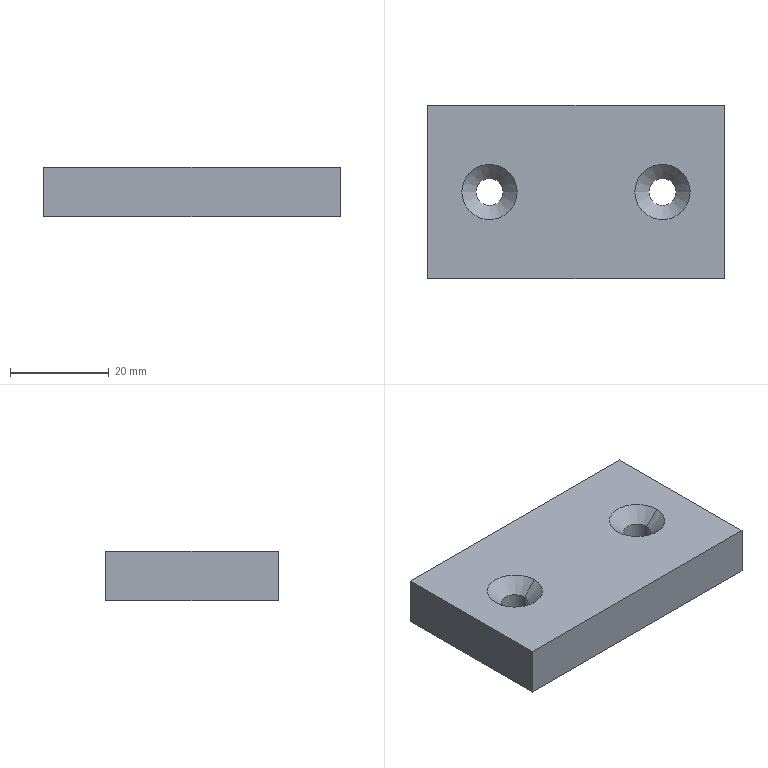Part | STEP file | 1 solid | 14 faces | box 60 x 35 x 10 mm | volume 20336 mm3 | plane 6 | cone 4 | cylinder 4 | commonest cylinder face diameters 5.5 x4
STEP:
#1=CARTESIAN_POINT('',(0.,0.,0.));
#2=DIRECTION('',(0.,0.,1.));
#3=DIRECTION('',(1.,0.,0.));
#4=AXIS2_PLACEMENT_3D('',#1,#2,#3);
#5=CARTESIAN_POINT('',(-14.75,0.,2.15));
#6=VERTEX_POINT('',#5);
#7=CARTESIAN_POINT('',(-11.9,0.,5.));
#8=VERTEX_POINT('',#7);
#9=CARTESIAN_POINT('',(-11.9,0.,5.));
#10=DIRECTION('',(0.7071,0.,0.7071));
#11=VECTOR('',#10,1.);
#12=LINE('',#9,#11);
#13=CARTESIAN_POINT('',(-17.5,0.,5.));
#14=DIRECTION('',(0.,0.,1.));
#15=DIRECTION('',(1.,0.,0.));
#16=AXIS2_PLACEMENT_3D('',#13,#14,#15);
#17=CONICAL_SURFACE('',#16,5.6,0.7854);
#18=CARTESIAN_POINT('',(6.283,0.));
#19=DIRECTION('',(0.,1.));
#20=VECTOR('',#19,1.);
#21=LINE('',#18,#20);
#22=(GEOMETRIC_REPRESENTATION_CONTEXT(2)PARAMETRIC_REPRESENTATION_CONTEXT()REPRESENTATION_CONTEXT('',''));
#23=DEFINITIONAL_REPRESENTATION('',(#21),#22);
#24=PCURVE('',#17,#23);
#25=CARTESIAN_POINT('',(-17.5,0.,5.));
#26=DIRECTION('',(0.,0.,1.));
#27=DIRECTION('',(1.,0.,0.));
#28=AXIS2_PLACEMENT_3D('',#25,#26,#27);
#29=CONICAL_SURFACE('',#28,5.6,0.7854);
#30=CARTESIAN_POINT('',(0.,0.));
#31=DIRECTION('',(0.,1.));
#32=VECTOR('',#31,1.);
#33=LINE('',#30,#32);
#34=(GEOMETRIC_REPRESENTATION_CONTEXT(2)PARAMETRIC_REPRESENTATION_CONTEXT()REPRESENTATION_CONTEXT('',''));
#35=DEFINITIONAL_REPRESENTATION('',(#33),#34);
#36=PCURVE('',#29,#35);
#37=SURFACE_CURVE('',#12,(#24,#36),.PCURVE_S1.);
#38=EDGE_CURVE('',#6,#8,#37,.T.);
#39=ORIENTED_EDGE('',*,*,#38,.T.);
#40=CARTESIAN_POINT('',(-23.1,0.,5.));
#41=VERTEX_POINT('',#40);
#42=CARTESIAN_POINT('',(-17.5,0.,5.));
#43=DIRECTION('',(0.,0.,1.));
#44=DIRECTION('',(1.,0.,0.));
#45=AXIS2_PLACEMENT_3D('',#42,#43,#44);
#46=CIRCLE('',#45,5.6);
#47=CARTESIAN_POINT('',(0.,0.));
#48=DIRECTION('',(1.,0.));
#49=VECTOR('',#48,1.);
#50=LINE('',#47,#49);
#51=(GEOMETRIC_REPRESENTATION_CONTEXT(2)PARAMETRIC_REPRESENTATION_CONTEXT()REPRESENTATION_CONTEXT('',''));
#52=DEFINITIONAL_REPRESENTATION('',(#50),#51);
#53=PCURVE('',#17,#52);
#54=CARTESIAN_POINT('',(0.,0.,5.));
#55=DIRECTION('',(0.,0.,-1.));
#56=DIRECTION('',(-1.,0.,0.));
#57=AXIS2_PLACEMENT_3D('',#54,#55,#56);
#58=PLANE('',#57);
#59=CARTESIAN_POINT('',(11.9,0.));
#60=CARTESIAN_POINT('',(11.9,9.699));
#61=CARTESIAN_POINT('',(20.3,4.85));
#62=CARTESIAN_POINT('',(28.7,0.));
#63=CARTESIAN_POINT('',(20.3,-4.85));
#64=CARTESIAN_POINT('',(11.9,-9.699));
#65=CARTESIAN_POINT('',(11.9,0.));
#66=(BOUNDED_CURVE()B_SPLINE_CURVE(2,(#59,#60,#61,#62,#63,#64,#65),.UNSPECIFIED.,.T.,.F.)B_SPLINE_CURVE_WITH_KNOTS((1,2,2,2,2,1),(-2.094,0.,2.094,4.189,6.283,8.378),.UNSPECIFIED.)CURVE()GEOMETRIC_REPRESENTATION_ITEM()RATIONAL_B_SPLINE_CURVE((1.,0.5,1.,0.5,1.,0.5,1.))REPRESENTATION_ITEM(''));
#67=(GEOMETRIC_REPRESENTATION_CONTEXT(2)PARAMETRIC_REPRESENTATION_CONTEXT()REPRESENTATION_CONTEXT('',''));
#68=DEFINITIONAL_REPRESENTATION('',(#66),#67);
#69=PCURVE('',#58,#68);
#70=SURFACE_CURVE('',#46,(#53,#69),.PCURVE_S1.);
#71=EDGE_CURVE('',#41,#8,#70,.T.);
#72=ORIENTED_EDGE('',*,*,#71,.F.);
#73=CARTESIAN_POINT('',(-20.25,0.,2.15));
#74=VERTEX_POINT('',#73);
#75=CARTESIAN_POINT('',(-23.1,0.,5.));
#76=DIRECTION('',(-0.7071,0.,0.7071));
#77=VECTOR('',#76,1.);
#78=LINE('',#75,#77);
#79=CARTESIAN_POINT('',(3.142,0.));
#80=DIRECTION('',(0.,1.));
#81=VECTOR('',#80,1.);
#82=LINE('',#79,#81);
#83=(GEOMETRIC_REPRESENTATION_CONTEXT(2)PARAMETRIC_REPRESENTATION_CONTEXT()REPRESENTATION_CONTEXT('',''));
#84=DEFINITIONAL_REPRESENTATION('',(#82),#83);
#85=PCURVE('',#17,#84);
#86=CARTESIAN_POINT('',(3.142,0.));
#87=DIRECTION('',(0.,1.));
#88=VECTOR('',#87,1.);
#89=LINE('',#86,#88);
#90=(GEOMETRIC_REPRESENTATION_CONTEXT(2)PARAMETRIC_REPRESENTATION_CONTEXT()REPRESENTATION_CONTEXT('',''));
#91=DEFINITIONAL_REPRESENTATION('',(#89),#90);
#92=PCURVE('',#29,#91);
#93=SURFACE_CURVE('',#78,(#85,#92),.PCURVE_S1.);
#94=EDGE_CURVE('',#74,#41,#93,.T.);
#95=ORIENTED_EDGE('',*,*,#94,.F.);
#96=CARTESIAN_POINT('',(-17.5,0.,2.15));
#97=DIRECTION('',(0.,0.,1.));
#98=DIRECTION('',(1.,0.,0.));
#99=AXIS2_PLACEMENT_3D('',#96,#97,#98);
#100=CIRCLE('',#99,2.75);
#101=CARTESIAN_POINT('',(0.,-2.85));
#102=DIRECTION('',(1.,0.));
#103=VECTOR('',#102,1.);
#104=LINE('',#101,#103);
#105=(GEOMETRIC_REPRESENTATION_CONTEXT(2)PARAMETRIC_REPRESENTATION_CONTEXT()REPRESENTATION_CONTEXT('',''));
#106=DEFINITIONAL_REPRESENTATION('',(#104),#105);
#107=PCURVE('',#17,#106);
#108=CARTESIAN_POINT('',(-17.5,0.,5.));
#109=DIRECTION('',(0.,0.,1.));
#110=DIRECTION('',(1.,0.,0.));
#111=AXIS2_PLACEMENT_3D('',#108,#109,#110);
#112=CYLINDRICAL_SURFACE('',#111,2.75);
#113=CARTESIAN_POINT('',(0.,-2.85));
#114=DIRECTION('',(1.,0.));
#115=VECTOR('',#114,1.);
#116=LINE('',#113,#115);
#117=(GEOMETRIC_REPRESENTATION_CONTEXT(2)PARAMETRIC_REPRESENTATION_CONTEXT()REPRESENTATION_CONTEXT('',''));
#118=DEFINITIONAL_REPRESENTATION('',(#116),#117);
#119=PCURVE('',#112,#118);
#120=SURFACE_CURVE('',#100,(#107,#119),.PCURVE_S1.);
#121=EDGE_CURVE('',#74,#6,#120,.T.);
#122=ORIENTED_EDGE('',*,*,#121,.T.);
#123=EDGE_LOOP('',(#39,#72,#95,#122));
#124=FACE_BOUND('',#123,.F.);
#125=ADVANCED_FACE('',(#124),#17,.F.);
#126=CARTESIAN_POINT('',(-14.75,0.,-5.));
#127=VERTEX_POINT('',#126);
#128=CARTESIAN_POINT('',(-14.75,0.,5.));
#129=DIRECTION('',(0.,0.,1.));
#130=VECTOR('',#129,1.);
#131=LINE('',#128,#130);
#132=CARTESIAN_POINT('',(6.283,0.));
#133=DIRECTION('',(0.,1.));
#134=VECTOR('',#133,1.);
#135=LINE('',#132,#134);
#136=(GEOMETRIC_REPRESENTATION_CONTEXT(2)PARAMETRIC_REPRESENTATION_CONTEXT()REPRESENTATION_CONTEXT('',''));
#137=DEFINITIONAL_REPRESENTATION('',(#135),#136);
#138=PCURVE('',#112,#137);
#139=CARTESIAN_POINT('',(-17.5,0.,5.));
#140=DIRECTION('',(0.,0.,1.));
#141=DIRECTION('',(1.,0.,0.));
#142=AXIS2_PLACEMENT_3D('',#139,#140,#141);
#143=CYLINDRICAL_SURFACE('',#142,2.75);
#144=CARTESIAN_POINT('',(0.,0.));
#145=DIRECTION('',(0.,1.));
#146=VECTOR('',#145,1.);
#147=LINE('',#144,#146);
#148=(GEOMETRIC_REPRESENTATION_CONTEXT(2)PARAMETRIC_REPRESENTATION_CONTEXT()REPRESENTATION_CONTEXT('',''));
#149=DEFINITIONAL_REPRESENTATION('',(#147),#148);
#150=PCURVE('',#143,#149);
#151=SURFACE_CURVE('',#131,(#138,#150),.PCURVE_S1.);
#152=EDGE_CURVE('',#127,#6,#151,.T.);
#153=ORIENTED_EDGE('',*,*,#152,.T.);
#154=ORIENTED_EDGE('',*,*,#121,.F.);
#155=CARTESIAN_POINT('',(-20.25,0.,-5.));
#156=VERTEX_POINT('',#155);
#157=CARTESIAN_POINT('',(-20.25,0.,5.));
#158=DIRECTION('',(0.,0.,1.));
#159=VECTOR('',#158,1.);
#160=LINE('',#157,#159);
#161=CARTESIAN_POINT('',(3.142,0.));
#162=DIRECTION('',(0.,1.));
#163=VECTOR('',#162,1.);
#164=LINE('',#161,#163);
#165=(GEOMETRIC_REPRESENTATION_CONTEXT(2)PARAMETRIC_REPRESENTATION_CONTEXT()REPRESENTATION_CONTEXT('',''));
#166=DEFINITIONAL_REPRESENTATION('',(#164),#165);
#167=PCURVE('',#112,#166);
#168=CARTESIAN_POINT('',(3.142,0.));
#169=DIRECTION('',(0.,1.));
#170=VECTOR('',#169,1.);
#171=LINE('',#168,#170);
#172=(GEOMETRIC_REPRESENTATION_CONTEXT(2)PARAMETRIC_REPRESENTATION_CONTEXT()REPRESENTATION_CONTEXT('',''));
#173=DEFINITIONAL_REPRESENTATION('',(#171),#172);
#174=PCURVE('',#143,#173);
#175=SURFACE_CURVE('',#160,(#167,#174),.PCURVE_S1.);
#176=EDGE_CURVE('',#156,#74,#175,.T.);
#177=ORIENTED_EDGE('',*,*,#176,.F.);
#178=CARTESIAN_POINT('',(-17.5,0.,-5.));
#179=DIRECTION('',(0.,0.,1.));
#180=DIRECTION('',(1.,0.,0.));
#181=AXIS2_PLACEMENT_3D('',#178,#179,#180);
#182=CIRCLE('',#181,2.75);
#183=CARTESIAN_POINT('',(0.,-10.));
#184=DIRECTION('',(1.,0.));
#185=VECTOR('',#184,1.);
#186=LINE('',#183,#185);
#187=(GEOMETRIC_REPRESENTATION_CONTEXT(2)PARAMETRIC_REPRESENTATION_CONTEXT()REPRESENTATION_CONTEXT('',''));
#188=DEFINITIONAL_REPRESENTATION('',(#186),#187);
#189=PCURVE('',#112,#188);
#190=CARTESIAN_POINT('',(0.,0.,-5.));
#191=DIRECTION('',(0.,0.,-1.));
#192=DIRECTION('',(-1.,0.,0.));
#193=AXIS2_PLACEMENT_3D('',#190,#191,#192);
#194=PLANE('',#193);
#195=CARTESIAN_POINT('',(14.75,0.));
#196=CARTESIAN_POINT('',(14.75,4.763));
#197=CARTESIAN_POINT('',(18.875,2.382));
#198=CARTESIAN_POINT('',(23.,0.));
#199=CARTESIAN_POINT('',(18.875,-2.382));
#200=CARTESIAN_POINT('',(14.75,-4.763));
#201=CARTESIAN_POINT('',(14.75,0.));
#202=(BOUNDED_CURVE()B_SPLINE_CURVE(2,(#195,#196,#197,#198,#199,#200,#201),.UNSPECIFIED.,.T.,.F.)B_SPLINE_CURVE_WITH_KNOTS((1,2,2,2,2,1),(-2.094,0.,2.094,4.189,6.283,8.378),.UNSPECIFIED.)CURVE()GEOMETRIC_REPRESENTATION_ITEM()RATIONAL_B_SPLINE_CURVE((1.,0.5,1.,0.5,1.,0.5,1.))REPRESENTATION_ITEM(''));
#203=(GEOMETRIC_REPRESENTATION_CONTEXT(2)PARAMETRIC_REPRESENTATION_CONTEXT()REPRESENTATION_CONTEXT('',''));
#204=DEFINITIONAL_REPRESENTATION('',(#202),#203);
#205=PCURVE('',#194,#204);
#206=SURFACE_CURVE('',#182,(#189,#205),.PCURVE_S1.);
#207=EDGE_CURVE('',#156,#127,#206,.T.);
#208=ORIENTED_EDGE('',*,*,#207,.T.);
#209=EDGE_LOOP('',(#153,#154,#177,#208));
#210=FACE_BOUND('',#209,.F.);
#211=ADVANCED_FACE('',(#210),#112,.F.);
#212=CARTESIAN_POINT('',(20.25,0.,2.15));
#213=VERTEX_POINT('',#212);
#214=CARTESIAN_POINT('',(23.1,0.,5.));
#215=VERTEX_POINT('',#214);
#216=CARTESIAN_POINT('',(23.1,0.,5.));
#217=DIRECTION('',(0.7071,0.,0.7071));
#218=VECTOR('',#217,1.);
#219=LINE('',#216,#218);
#220=CARTESIAN_POINT('',(17.5,0.,5.));
#221=DIRECTION('',(0.,0.,1.));
#222=DIRECTION('',(1.,0.,0.));
#223=AXIS2_PLACEMENT_3D('',#220,#221,#222);
#224=CONICAL_SURFACE('',#223,5.6,0.7854);
#225=CARTESIAN_POINT('',(6.283,0.));
#226=DIRECTION('',(0.,1.));
#227=VECTOR('',#226,1.);
#228=LINE('',#225,#227);
#229=(GEOMETRIC_REPRESENTATION_CONTEXT(2)PARAMETRIC_REPRESENTATION_CONTEXT()REPRESENTATION_CONTEXT('',''));
#230=DEFINITIONAL_REPRESENTATION('',(#228),#229);
#231=PCURVE('',#224,#230);
#232=CARTESIAN_POINT('',(17.5,0.,5.));
#233=DIRECTION('',(0.,0.,1.));
#234=DIRECTION('',(1.,0.,0.));
#235=AXIS2_PLACEMENT_3D('',#232,#233,#234);
#236=CONICAL_SURFACE('',#235,5.6,0.7854);
#237=CARTESIAN_POINT('',(0.,0.));
#238=DIRECTION('',(0.,1.));
#239=VECTOR('',#238,1.);
#240=LINE('',#237,#239);
#241=(GEOMETRIC_REPRESENTATION_CONTEXT(2)PARAMETRIC_REPRESENTATION_CONTEXT()REPRESENTATION_CONTEXT('',''));
#242=DEFINITIONAL_REPRESENTATION('',(#240),#241);
#243=PCURVE('',#236,#242);
#244=SURFACE_CURVE('',#219,(#231,#243),.PCURVE_S1.);
#245=EDGE_CURVE('',#213,#215,#244,.T.);
#246=ORIENTED_EDGE('',*,*,#245,.T.);
#247=CARTESIAN_POINT('',(11.9,0.,5.));
#248=VERTEX_POINT('',#247);
#249=CARTESIAN_POINT('',(17.5,0.,5.));
#250=DIRECTION('',(0.,0.,1.));
#251=DIRECTION('',(1.,0.,0.));
#252=AXIS2_PLACEMENT_3D('',#249,#250,#251);
#253=CIRCLE('',#252,5.6);
#254=CARTESIAN_POINT('',(0.,0.));
#255=DIRECTION('',(1.,0.));
#256=VECTOR('',#255,1.);
#257=LINE('',#254,#256);
#258=(GEOMETRIC_REPRESENTATION_CONTEXT(2)PARAMETRIC_REPRESENTATION_CONTEXT()REPRESENTATION_CONTEXT('',''));
#259=DEFINITIONAL_REPRESENTATION('',(#257),#258);
#260=PCURVE('',#224,#259);
#261=CARTESIAN_POINT('',(-23.1,0.));
#262=CARTESIAN_POINT('',(-23.1,9.699));
#263=CARTESIAN_POINT('',(-14.7,4.85));
#264=CARTESIAN_POINT('',(-6.3,0.));
#265=CARTESIAN_POINT('',(-14.7,-4.85));
#266=CARTESIAN_POINT('',(-23.1,-9.699));
#267=CARTESIAN_POINT('',(-23.1,0.));
#268=(BOUNDED_CURVE()B_SPLINE_CURVE(2,(#261,#262,#263,#264,#265,#266,#267),.UNSPECIFIED.,.T.,.F.)B_SPLINE_CURVE_WITH_KNOTS((1,2,2,2,2,1),(-2.094,0.,2.094,4.189,6.283,8.378),.UNSPECIFIED.)CURVE()GEOMETRIC_REPRESENTATION_ITEM()RATIONAL_B_SPLINE_CURVE((1.,0.5,1.,0.5,1.,0.5,1.))REPRESENTATION_ITEM(''));
#269=(GEOMETRIC_REPRESENTATION_CONTEXT(2)PARAMETRIC_REPRESENTATION_CONTEXT()REPRESENTATION_CONTEXT('',''));
#270=DEFINITIONAL_REPRESENTATION('',(#268),#269);
#271=PCURVE('',#58,#270);
#272=SURFACE_CURVE('',#253,(#260,#271),.PCURVE_S1.);
#273=EDGE_CURVE('',#248,#215,#272,.T.);
#274=ORIENTED_EDGE('',*,*,#273,.F.);
#275=CARTESIAN_POINT('',(14.75,0.,2.15));
#276=VERTEX_POINT('',#275);
#277=CARTESIAN_POINT('',(11.9,0.,5.));
#278=DIRECTION('',(-0.7071,0.,0.7071));
#279=VECTOR('',#278,1.);
#280=LINE('',#277,#279);
#281=CARTESIAN_POINT('',(3.142,0.));
#282=DIRECTION('',(0.,1.));
#283=VECTOR('',#282,1.);
#284=LINE('',#281,#283);
#285=(GEOMETRIC_REPRESENTATION_CONTEXT(2)PARAMETRIC_REPRESENTATION_CONTEXT()REPRESENTATION_CONTEXT('',''));
#286=DEFINITIONAL_REPRESENTATION('',(#284),#285);
#287=PCURVE('',#224,#286);
#288=CARTESIAN_POINT('',(3.142,0.));
#289=DIRECTION('',(0.,1.));
#290=VECTOR('',#289,1.);
#291=LINE('',#288,#290);
#292=(GEOMETRIC_REPRESENTATION_CONTEXT(2)PARAMETRIC_REPRESENTATION_CONTEXT()REPRESENTATION_CONTEXT('',''));
#293=DEFINITIONAL_REPRESENTATION('',(#291),#292);
#294=PCURVE('',#236,#293);
#295=SURFACE_CURVE('',#280,(#287,#294),.PCURVE_S1.);
#296=EDGE_CURVE('',#276,#248,#295,.T.);
#297=ORIENTED_EDGE('',*,*,#296,.F.);
#298=CARTESIAN_POINT('',(17.5,0.,2.15));
#299=DIRECTION('',(0.,0.,1.));
#300=DIRECTION('',(1.,0.,0.));
#301=AXIS2_PLACEMENT_3D('',#298,#299,#300);
#302=CIRCLE('',#301,2.75);
#303=CARTESIAN_POINT('',(0.,-2.85));
#304=DIRECTION('',(1.,0.));
#305=VECTOR('',#304,1.);
#306=LINE('',#303,#305);
#307=(GEOMETRIC_REPRESENTATION_CONTEXT(2)PARAMETRIC_REPRESENTATION_CONTEXT()REPRESENTATION_CONTEXT('',''));
#308=DEFINITIONAL_REPRESENTATION('',(#306),#307);
#309=PCURVE('',#224,#308);
#310=CARTESIAN_POINT('',(17.5,0.,5.));
#311=DIRECTION('',(0.,0.,1.));
#312=DIRECTION('',(1.,0.,0.));
#313=AXIS2_PLACEMENT_3D('',#310,#311,#312);
#314=CYLINDRICAL_SURFACE('',#313,2.75);
#315=CARTESIAN_POINT('',(0.,-2.85));
#316=DIRECTION('',(1.,0.));
#317=VECTOR('',#316,1.);
#318=LINE('',#315,#317);
#319=(GEOMETRIC_REPRESENTATION_CONTEXT(2)PARAMETRIC_REPRESENTATION_CONTEXT()REPRESENTATION_CONTEXT('',''));
#320=DEFINITIONAL_REPRESENTATION('',(#318),#319);
#321=PCURVE('',#314,#320);
#322=SURFACE_CURVE('',#302,(#309,#321),.PCURVE_S1.);
#323=EDGE_CURVE('',#276,#213,#322,.T.);
#324=ORIENTED_EDGE('',*,*,#323,.T.);
#325=EDGE_LOOP('',(#246,#274,#297,#324));
#326=FACE_BOUND('',#325,.F.);
#327=ADVANCED_FACE('',(#326),#224,.F.);
#328=CARTESIAN_POINT('',(20.25,0.,-5.));
#329=VERTEX_POINT('',#328);
#330=CARTESIAN_POINT('',(20.25,0.,5.));
#331=DIRECTION('',(0.,0.,1.));
#332=VECTOR('',#331,1.);
#333=LINE('',#330,#332);
#334=CARTESIAN_POINT('',(6.283,0.));
#335=DIRECTION('',(0.,1.));
#336=VECTOR('',#335,1.);
#337=LINE('',#334,#336);
#338=(GEOMETRIC_REPRESENTATION_CONTEXT(2)PARAMETRIC_REPRESENTATION_CONTEXT()REPRESENTATION_CONTEXT('',''));
#339=DEFINITIONAL_REPRESENTATION('',(#337),#338);
#340=PCURVE('',#314,#339);
#341=CARTESIAN_POINT('',(17.5,0.,5.));
#342=DIRECTION('',(0.,0.,1.));
#343=DIRECTION('',(1.,0.,0.));
#344=AXIS2_PLACEMENT_3D('',#341,#342,#343);
#345=CYLINDRICAL_SURFACE('',#344,2.75);
#346=CARTESIAN_POINT('',(0.,0.));
#347=DIRECTION('',(0.,1.));
#348=VECTOR('',#347,1.);
#349=LINE('',#346,#348);
#350=(GEOMETRIC_REPRESENTATION_CONTEXT(2)PARAMETRIC_REPRESENTATION_CONTEXT()REPRESENTATION_CONTEXT('',''));
#351=DEFINITIONAL_REPRESENTATION('',(#349),#350);
#352=PCURVE('',#345,#351);
#353=SURFACE_CURVE('',#333,(#340,#352),.PCURVE_S1.);
#354=EDGE_CURVE('',#329,#213,#353,.T.);
#355=ORIENTED_EDGE('',*,*,#354,.T.);
#356=ORIENTED_EDGE('',*,*,#323,.F.);
#357=CARTESIAN_POINT('',(14.75,0.,-5.));
#358=VERTEX_POINT('',#357);
#359=CARTESIAN_POINT('',(14.75,0.,5.));
#360=DIRECTION('',(0.,0.,1.));
#361=VECTOR('',#360,1.);
#362=LINE('',#359,#361);
#363=CARTESIAN_POINT('',(3.142,0.));
#364=DIRECTION('',(0.,1.));
#365=VECTOR('',#364,1.);
#366=LINE('',#363,#365);
#367=(GEOMETRIC_REPRESENTATION_CONTEXT(2)PARAMETRIC_REPRESENTATION_CONTEXT()REPRESENTATION_CONTEXT('',''));
#368=DEFINITIONAL_REPRESENTATION('',(#366),#367);
#369=PCURVE('',#314,#368);
#370=CARTESIAN_POINT('',(3.142,0.));
#371=DIRECTION('',(0.,1.));
#372=VECTOR('',#371,1.);
#373=LINE('',#370,#372);
#374=(GEOMETRIC_REPRESENTATION_CONTEXT(2)PARAMETRIC_REPRESENTATION_CONTEXT()REPRESENTATION_CONTEXT('',''));
#375=DEFINITIONAL_REPRESENTATION('',(#373),#374);
#376=PCURVE('',#345,#375);
#377=SURFACE_CURVE('',#362,(#369,#376),.PCURVE_S1.);
#378=EDGE_CURVE('',#358,#276,#377,.T.);
#379=ORIENTED_EDGE('',*,*,#378,.F.);
#380=CARTESIAN_POINT('',(17.5,0.,-5.));
#381=DIRECTION('',(0.,0.,1.));
#382=DIRECTION('',(1.,0.,0.));
#383=AXIS2_PLACEMENT_3D('',#380,#381,#382);
#384=CIRCLE('',#383,2.75);
#385=CARTESIAN_POINT('',(0.,-10.));
#386=DIRECTION('',(1.,0.));
#387=VECTOR('',#386,1.);
#388=LINE('',#385,#387);
#389=(GEOMETRIC_REPRESENTATION_CONTEXT(2)PARAMETRIC_REPRESENTATION_CONTEXT()REPRESENTATION_CONTEXT('',''));
#390=DEFINITIONAL_REPRESENTATION('',(#388),#389);
#391=PCURVE('',#314,#390);
#392=CARTESIAN_POINT('',(-20.25,0.));
#393=CARTESIAN_POINT('',(-20.25,4.763));
#394=CARTESIAN_POINT('',(-16.125,2.382));
#395=CARTESIAN_POINT('',(-12.,0.));
#396=CARTESIAN_POINT('',(-16.125,-2.382));
#397=CARTESIAN_POINT('',(-20.25,-4.763));
#398=CARTESIAN_POINT('',(-20.25,0.));
#399=(BOUNDED_CURVE()B_SPLINE_CURVE(2,(#392,#393,#394,#395,#396,#397,#398),.UNSPECIFIED.,.T.,.F.)B_SPLINE_CURVE_WITH_KNOTS((1,2,2,2,2,1),(-2.094,0.,2.094,4.189,6.283,8.378),.UNSPECIFIED.)CURVE()GEOMETRIC_REPRESENTATION_ITEM()RATIONAL_B_SPLINE_CURVE((1.,0.5,1.,0.5,1.,0.5,1.))REPRESENTATION_ITEM(''));
#400=(GEOMETRIC_REPRESENTATION_CONTEXT(2)PARAMETRIC_REPRESENTATION_CONTEXT()REPRESENTATION_CONTEXT('',''));
#401=DEFINITIONAL_REPRESENTATION('',(#399),#400);
#402=PCURVE('',#194,#401);
#403=SURFACE_CURVE('',#384,(#391,#402),.PCURVE_S1.);
#404=EDGE_CURVE('',#358,#329,#403,.T.);
#405=ORIENTED_EDGE('',*,*,#404,.T.);
#406=EDGE_LOOP('',(#355,#356,#379,#405));
#407=FACE_BOUND('',#406,.F.);
#408=ADVANCED_FACE('',(#407),#314,.F.);
#409=CARTESIAN_POINT('',(30.,-17.5,-5.));
#410=VERTEX_POINT('',#409);
#411=CARTESIAN_POINT('',(30.,17.5,-5.));
#412=VERTEX_POINT('',#411);
#413=CARTESIAN_POINT('',(30.,-17.5,-5.));
#414=DIRECTION('',(0.,1.,0.));
#415=VECTOR('',#414,1.);
#416=LINE('',#413,#415);
#417=CARTESIAN_POINT('',(30.,-17.5,5.));
#418=DIRECTION('',(-1.,0.,0.));
#419=DIRECTION('',(0.,0.,1.));
#420=AXIS2_PLACEMENT_3D('',#417,#418,#419);
#421=PLANE('',#420);
#422=CARTESIAN_POINT('',(-10.,0.));
#423=DIRECTION('',(0.,1.));
#424=VECTOR('',#423,1.);
#425=LINE('',#422,#424);
#426=(GEOMETRIC_REPRESENTATION_CONTEXT(2)PARAMETRIC_REPRESENTATION_CONTEXT()REPRESENTATION_CONTEXT('',''));
#427=DEFINITIONAL_REPRESENTATION('',(#425),#426);
#428=PCURVE('',#421,#427);
#429=CARTESIAN_POINT('',(-30.,-17.5));
#430=DIRECTION('',(0.,1.));
#431=VECTOR('',#430,1.);
#432=LINE('',#429,#431);
#433=(GEOMETRIC_REPRESENTATION_CONTEXT(2)PARAMETRIC_REPRESENTATION_CONTEXT()REPRESENTATION_CONTEXT('',''));
#434=DEFINITIONAL_REPRESENTATION('',(#432),#433);
#435=PCURVE('',#194,#434);
#436=SURFACE_CURVE('',#416,(#428,#435),.PCURVE_S1.);
#437=EDGE_CURVE('',#410,#412,#436,.T.);
#438=ORIENTED_EDGE('',*,*,#437,.T.);
#439=CARTESIAN_POINT('',(30.,17.5,5.));
#440=VERTEX_POINT('',#439);
#441=CARTESIAN_POINT('',(30.,17.5,5.));
#442=DIRECTION('',(0.,0.,-1.));
#443=VECTOR('',#442,1.);
#444=LINE('',#441,#443);
#445=CARTESIAN_POINT('',(0.,35.));
#446=DIRECTION('',(-1.,0.));
#447=VECTOR('',#446,1.);
#448=LINE('',#445,#447);
#449=(GEOMETRIC_REPRESENTATION_CONTEXT(2)PARAMETRIC_REPRESENTATION_CONTEXT()REPRESENTATION_CONTEXT('',''));
#450=DEFINITIONAL_REPRESENTATION('',(#448),#449);
#451=PCURVE('',#421,#450);
#452=CARTESIAN_POINT('',(-30.,17.5,5.));
#453=DIRECTION('',(0.,-1.,0.));
#454=DIRECTION('',(0.,0.,-1.));
#455=AXIS2_PLACEMENT_3D('',#452,#453,#454);
#456=PLANE('',#455);
#457=CARTESIAN_POINT('',(0.,60.));
#458=DIRECTION('',(1.,0.));
#459=VECTOR('',#458,1.);
#460=LINE('',#457,#459);
#461=(GEOMETRIC_REPRESENTATION_CONTEXT(2)PARAMETRIC_REPRESENTATION_CONTEXT()REPRESENTATION_CONTEXT('',''));
#462=DEFINITIONAL_REPRESENTATION('',(#460),#461);
#463=PCURVE('',#456,#462);
#464=SURFACE_CURVE('',#444,(#451,#463),.PCURVE_S1.);
#465=EDGE_CURVE('',#440,#412,#464,.T.);
#466=ORIENTED_EDGE('',*,*,#465,.F.);
#467=CARTESIAN_POINT('',(30.,-17.5,5.));
#468=VERTEX_POINT('',#467);
#469=CARTESIAN_POINT('',(30.,-17.5,5.));
#470=DIRECTION('',(0.,1.,0.));
#471=VECTOR('',#470,1.);
#472=LINE('',#469,#471);
#473=CARTESIAN_POINT('',(0.,0.));
#474=DIRECTION('',(0.,1.));
#475=VECTOR('',#474,1.);
#476=LINE('',#473,#475);
#477=(GEOMETRIC_REPRESENTATION_CONTEXT(2)PARAMETRIC_REPRESENTATION_CONTEXT()REPRESENTATION_CONTEXT('',''));
#478=DEFINITIONAL_REPRESENTATION('',(#476),#477);
#479=PCURVE('',#421,#478);
#480=CARTESIAN_POINT('',(-30.,-17.5));
#481=DIRECTION('',(0.,1.));
#482=VECTOR('',#481,1.);
#483=LINE('',#480,#482);
#484=(GEOMETRIC_REPRESENTATION_CONTEXT(2)PARAMETRIC_REPRESENTATION_CONTEXT()REPRESENTATION_CONTEXT('',''));
#485=DEFINITIONAL_REPRESENTATION('',(#483),#484);
#486=PCURVE('',#58,#485);
#487=SURFACE_CURVE('',#472,(#479,#486),.PCURVE_S1.);
#488=EDGE_CURVE('',#468,#440,#487,.T.);
#489=ORIENTED_EDGE('',*,*,#488,.F.);
#490=CARTESIAN_POINT('',(30.,-17.5,5.));
#491=DIRECTION('',(0.,0.,-1.));
#492=VECTOR('',#491,1.);
#493=LINE('',#490,#492);
#494=CARTESIAN_POINT('',(0.,0.));
#495=DIRECTION('',(-1.,0.));
#496=VECTOR('',#495,1.);
#497=LINE('',#494,#496);
#498=(GEOMETRIC_REPRESENTATION_CONTEXT(2)PARAMETRIC_REPRESENTATION_CONTEXT()REPRESENTATION_CONTEXT('',''));
#499=DEFINITIONAL_REPRESENTATION('',(#497),#498);
#500=PCURVE('',#421,#499);
#501=CARTESIAN_POINT('',(-30.,-17.5,5.));
#502=DIRECTION('',(0.,1.,0.));
#503=DIRECTION('',(0.,0.,1.));
#504=AXIS2_PLACEMENT_3D('',#501,#502,#503);
#505=PLANE('',#504);
#506=CARTESIAN_POINT('',(0.,60.));
#507=DIRECTION('',(-1.,0.));
#508=VECTOR('',#507,1.);
#509=LINE('',#506,#508);
#510=(GEOMETRIC_REPRESENTATION_CONTEXT(2)PARAMETRIC_REPRESENTATION_CONTEXT()REPRESENTATION_CONTEXT('',''));
#511=DEFINITIONAL_REPRESENTATION('',(#509),#510);
#512=PCURVE('',#505,#511);
#513=SURFACE_CURVE('',#493,(#500,#512),.PCURVE_S1.);
#514=EDGE_CURVE('',#468,#410,#513,.T.);
#515=ORIENTED_EDGE('',*,*,#514,.T.);
#516=EDGE_LOOP('',(#438,#466,#489,#515));
#517=FACE_BOUND('',#516,.T.);
#518=ADVANCED_FACE('',(#517),#421,.F.);
#519=CARTESIAN_POINT('',(-30.,17.5,-5.));
#520=VERTEX_POINT('',#519);
#521=CARTESIAN_POINT('',(-30.,17.5,-5.));
#522=DIRECTION('',(-1.,0.,0.));
#523=VECTOR('',#522,1.);
#524=LINE('',#521,#523);
#525=CARTESIAN_POINT('',(10.,0.));
#526=DIRECTION('',(0.,-1.));
#527=VECTOR('',#526,1.);
#528=LINE('',#525,#527);
#529=(GEOMETRIC_REPRESENTATION_CONTEXT(2)PARAMETRIC_REPRESENTATION_CONTEXT()REPRESENTATION_CONTEXT('',''));
#530=DEFINITIONAL_REPRESENTATION('',(#528),#529);
#531=PCURVE('',#456,#530);
#532=CARTESIAN_POINT('',(30.,17.5));
#533=DIRECTION('',(1.,0.));
#534=VECTOR('',#533,1.);
#535=LINE('',#532,#534);
#536=(GEOMETRIC_REPRESENTATION_CONTEXT(2)PARAMETRIC_REPRESENTATION_CONTEXT()REPRESENTATION_CONTEXT('',''));
#537=DEFINITIONAL_REPRESENTATION('',(#535),#536);
#538=PCURVE('',#194,#537);
#539=SURFACE_CURVE('',#524,(#531,#538),.PCURVE_S1.);
#540=EDGE_CURVE('',#412,#520,#539,.T.);
#541=ORIENTED_EDGE('',*,*,#540,.T.);
#542=CARTESIAN_POINT('',(-30.,17.5,5.));
#543=VERTEX_POINT('',#542);
#544=CARTESIAN_POINT('',(-30.,17.5,5.));
#545=DIRECTION('',(0.,0.,-1.));
#546=VECTOR('',#545,1.);
#547=LINE('',#544,#546);
#548=CARTESIAN_POINT('',(0.,0.));
#549=DIRECTION('',(1.,0.));
#550=VECTOR('',#549,1.);
#551=LINE('',#548,#550);
#552=(GEOMETRIC_REPRESENTATION_CONTEXT(2)PARAMETRIC_REPRESENTATION_CONTEXT()REPRESENTATION_CONTEXT('',''));
#553=DEFINITIONAL_REPRESENTATION('',(#551),#552);
#554=PCURVE('',#456,#553);
#555=CARTESIAN_POINT('',(-30.,-17.5,5.));
#556=DIRECTION('',(1.,0.,0.));
#557=DIRECTION('',(0.,0.,-1.));
#558=AXIS2_PLACEMENT_3D('',#555,#556,#557);
#559=PLANE('',#558);
#560=CARTESIAN_POINT('',(0.,35.));
#561=DIRECTION('',(1.,0.));
#562=VECTOR('',#561,1.);
#563=LINE('',#560,#562);
#564=(GEOMETRIC_REPRESENTATION_CONTEXT(2)PARAMETRIC_REPRESENTATION_CONTEXT()REPRESENTATION_CONTEXT('',''));
#565=DEFINITIONAL_REPRESENTATION('',(#563),#564);
#566=PCURVE('',#559,#565);
#567=SURFACE_CURVE('',#547,(#554,#566),.PCURVE_S1.);
#568=EDGE_CURVE('',#543,#520,#567,.T.);
#569=ORIENTED_EDGE('',*,*,#568,.F.);
#570=CARTESIAN_POINT('',(-30.,17.5,5.));
#571=DIRECTION('',(-1.,0.,0.));
#572=VECTOR('',#571,1.);
#573=LINE('',#570,#572);
#574=CARTESIAN_POINT('',(0.,0.));
#575=DIRECTION('',(0.,-1.));
#576=VECTOR('',#575,1.);
#577=LINE('',#574,#576);
#578=(GEOMETRIC_REPRESENTATION_CONTEXT(2)PARAMETRIC_REPRESENTATION_CONTEXT()REPRESENTATION_CONTEXT('',''));
#579=DEFINITIONAL_REPRESENTATION('',(#577),#578);
#580=PCURVE('',#456,#579);
#581=CARTESIAN_POINT('',(30.,17.5));
#582=DIRECTION('',(1.,0.));
#583=VECTOR('',#582,1.);
#584=LINE('',#581,#583);
#585=(GEOMETRIC_REPRESENTATION_CONTEXT(2)PARAMETRIC_REPRESENTATION_CONTEXT()REPRESENTATION_CONTEXT('',''));
#586=DEFINITIONAL_REPRESENTATION('',(#584),#585);
#587=PCURVE('',#58,#586);
#588=SURFACE_CURVE('',#573,(#580,#587),.PCURVE_S1.);
#589=EDGE_CURVE('',#440,#543,#588,.T.);
#590=ORIENTED_EDGE('',*,*,#589,.F.);
#591=ORIENTED_EDGE('',*,*,#465,.T.);
#592=EDGE_LOOP('',(#541,#569,#590,#591));
#593=FACE_BOUND('',#592,.T.);
#594=ADVANCED_FACE('',(#593),#456,.F.);
#595=CARTESIAN_POINT('',(-30.,-17.5,-5.));
#596=VERTEX_POINT('',#595);
#597=CARTESIAN_POINT('',(-30.,-17.5,-5.));
#598=DIRECTION('',(0.,-1.,0.));
#599=VECTOR('',#598,1.);
#600=LINE('',#597,#599);
#601=CARTESIAN_POINT('',(10.,0.));
#602=DIRECTION('',(0.,-1.));
#603=VECTOR('',#602,1.);
#604=LINE('',#601,#603);
#605=(GEOMETRIC_REPRESENTATION_CONTEXT(2)PARAMETRIC_REPRESENTATION_CONTEXT()REPRESENTATION_CONTEXT('',''));
#606=DEFINITIONAL_REPRESENTATION('',(#604),#605);
#607=PCURVE('',#559,#606);
#608=CARTESIAN_POINT('',(30.,-17.5));
#609=DIRECTION('',(0.,-1.));
#610=VECTOR('',#609,1.);
#611=LINE('',#608,#610);
#612=(GEOMETRIC_REPRESENTATION_CONTEXT(2)PARAMETRIC_REPRESENTATION_CONTEXT()REPRESENTATION_CONTEXT('',''));
#613=DEFINITIONAL_REPRESENTATION('',(#611),#612);
#614=PCURVE('',#194,#613);
#615=SURFACE_CURVE('',#600,(#607,#614),.PCURVE_S1.);
#616=EDGE_CURVE('',#520,#596,#615,.T.);
#617=ORIENTED_EDGE('',*,*,#616,.T.);
#618=CARTESIAN_POINT('',(-30.,-17.5,5.));
#619=VERTEX_POINT('',#618);
#620=CARTESIAN_POINT('',(-30.,-17.5,5.));
#621=DIRECTION('',(0.,0.,-1.));
#622=VECTOR('',#621,1.);
#623=LINE('',#620,#622);
#624=CARTESIAN_POINT('',(0.,0.));
#625=DIRECTION('',(1.,0.));
#626=VECTOR('',#625,1.);
#627=LINE('',#624,#626);
#628=(GEOMETRIC_REPRESENTATION_CONTEXT(2)PARAMETRIC_REPRESENTATION_CONTEXT()REPRESENTATION_CONTEXT('',''));
#629=DEFINITIONAL_REPRESENTATION('',(#627),#628);
#630=PCURVE('',#559,#629);
#631=CARTESIAN_POINT('',(0.,0.));
#632=DIRECTION('',(-1.,0.));
#633=VECTOR('',#632,1.);
#634=LINE('',#631,#633);
#635=(GEOMETRIC_REPRESENTATION_CONTEXT(2)PARAMETRIC_REPRESENTATION_CONTEXT()REPRESENTATION_CONTEXT('',''));
#636=DEFINITIONAL_REPRESENTATION('',(#634),#635);
#637=PCURVE('',#505,#636);
#638=SURFACE_CURVE('',#623,(#630,#637),.PCURVE_S1.);
#639=EDGE_CURVE('',#619,#596,#638,.T.);
#640=ORIENTED_EDGE('',*,*,#639,.F.);
#641=CARTESIAN_POINT('',(-30.,-17.5,5.));
#642=DIRECTION('',(0.,-1.,0.));
#643=VECTOR('',#642,1.);
#644=LINE('',#641,#643);
#645=CARTESIAN_POINT('',(0.,0.));
#646=DIRECTION('',(0.,-1.));
#647=VECTOR('',#646,1.);
#648=LINE('',#645,#647);
#649=(GEOMETRIC_REPRESENTATION_CONTEXT(2)PARAMETRIC_REPRESENTATION_CONTEXT()REPRESENTATION_CONTEXT('',''));
#650=DEFINITIONAL_REPRESENTATION('',(#648),#649);
#651=PCURVE('',#559,#650);
#652=CARTESIAN_POINT('',(30.,-17.5));
#653=DIRECTION('',(0.,-1.));
#654=VECTOR('',#653,1.);
#655=LINE('',#652,#654);
#656=(GEOMETRIC_REPRESENTATION_CONTEXT(2)PARAMETRIC_REPRESENTATION_CONTEXT()REPRESENTATION_CONTEXT('',''));
#657=DEFINITIONAL_REPRESENTATION('',(#655),#656);
#658=PCURVE('',#58,#657);
#659=SURFACE_CURVE('',#644,(#651,#658),.PCURVE_S1.);
#660=EDGE_CURVE('',#543,#619,#659,.T.);
#661=ORIENTED_EDGE('',*,*,#660,.F.);
#662=ORIENTED_EDGE('',*,*,#568,.T.);
#663=EDGE_LOOP('',(#617,#640,#661,#662));
#664=FACE_BOUND('',#663,.T.);
#665=ADVANCED_FACE('',(#664),#559,.F.);
#666=CARTESIAN_POINT('',(-30.,-17.5,-5.));
#667=DIRECTION('',(1.,0.,0.));
#668=VECTOR('',#667,1.);
#669=LINE('',#666,#668);
#670=CARTESIAN_POINT('',(-10.,0.));
#671=DIRECTION('',(0.,1.));
#672=VECTOR('',#671,1.);
#673=LINE('',#670,#672);
#674=(GEOMETRIC_REPRESENTATION_CONTEXT(2)PARAMETRIC_REPRESENTATION_CONTEXT()REPRESENTATION_CONTEXT('',''));
#675=DEFINITIONAL_REPRESENTATION('',(#673),#674);
#676=PCURVE('',#505,#675);
#677=CARTESIAN_POINT('',(30.,-17.5));
#678=DIRECTION('',(-1.,0.));
#679=VECTOR('',#678,1.);
#680=LINE('',#677,#679);
#681=(GEOMETRIC_REPRESENTATION_CONTEXT(2)PARAMETRIC_REPRESENTATION_CONTEXT()REPRESENTATION_CONTEXT('',''));
#682=DEFINITIONAL_REPRESENTATION('',(#680),#681);
#683=PCURVE('',#194,#682);
#684=SURFACE_CURVE('',#669,(#676,#683),.PCURVE_S1.);
#685=EDGE_CURVE('',#596,#410,#684,.T.);
#686=ORIENTED_EDGE('',*,*,#685,.T.);
#687=ORIENTED_EDGE('',*,*,#514,.F.);
#688=CARTESIAN_POINT('',(-30.,-17.5,5.));
#689=DIRECTION('',(1.,0.,0.));
#690=VECTOR('',#689,1.);
#691=LINE('',#688,#690);
#692=CARTESIAN_POINT('',(0.,0.));
#693=DIRECTION('',(0.,1.));
#694=VECTOR('',#693,1.);
#695=LINE('',#692,#694);
#696=(GEOMETRIC_REPRESENTATION_CONTEXT(2)PARAMETRIC_REPRESENTATION_CONTEXT()REPRESENTATION_CONTEXT('',''));
#697=DEFINITIONAL_REPRESENTATION('',(#695),#696);
#698=PCURVE('',#505,#697);
#699=CARTESIAN_POINT('',(30.,-17.5));
#700=DIRECTION('',(-1.,0.));
#701=VECTOR('',#700,1.);
#702=LINE('',#699,#701);
#703=(GEOMETRIC_REPRESENTATION_CONTEXT(2)PARAMETRIC_REPRESENTATION_CONTEXT()REPRESENTATION_CONTEXT('',''));
#704=DEFINITIONAL_REPRESENTATION('',(#702),#703);
#705=PCURVE('',#58,#704);
#706=SURFACE_CURVE('',#691,(#698,#705),.PCURVE_S1.);
#707=EDGE_CURVE('',#619,#468,#706,.T.);
#708=ORIENTED_EDGE('',*,*,#707,.F.);
#709=ORIENTED_EDGE('',*,*,#639,.T.);
#710=EDGE_LOOP('',(#686,#687,#708,#709));
#711=FACE_BOUND('',#710,.T.);
#712=ADVANCED_FACE('',(#711),#505,.F.);
#713=CARTESIAN_POINT('',(-17.5,0.,5.));
#714=DIRECTION('',(0.,0.,1.));
#715=DIRECTION('',(1.,0.,0.));
#716=AXIS2_PLACEMENT_3D('',#713,#714,#715);
#717=CIRCLE('',#716,5.6);
#718=CARTESIAN_POINT('',(11.9,0.));
#719=CARTESIAN_POINT('',(11.9,9.699));
#720=CARTESIAN_POINT('',(20.3,4.85));
#721=CARTESIAN_POINT('',(28.7,0.));
#722=CARTESIAN_POINT('',(20.3,-4.85));
#723=CARTESIAN_POINT('',(11.9,-9.699));
#724=CARTESIAN_POINT('',(11.9,0.));
#725=(BOUNDED_CURVE()B_SPLINE_CURVE(2,(#718,#719,#720,#721,#722,#723,#724),.UNSPECIFIED.,.T.,.F.)B_SPLINE_CURVE_WITH_KNOTS((1,2,2,2,2,1),(-2.094,0.,2.094,4.189,6.283,8.378),.UNSPECIFIED.)CURVE()GEOMETRIC_REPRESENTATION_ITEM()RATIONAL_B_SPLINE_CURVE((1.,0.5,1.,0.5,1.,0.5,1.))REPRESENTATION_ITEM(''));
#726=(GEOMETRIC_REPRESENTATION_CONTEXT(2)PARAMETRIC_REPRESENTATION_CONTEXT()REPRESENTATION_CONTEXT('',''));
#727=DEFINITIONAL_REPRESENTATION('',(#725),#726);
#728=PCURVE('',#58,#727);
#729=CARTESIAN_POINT('',(0.,0.));
#730=DIRECTION('',(1.,0.));
#731=VECTOR('',#730,1.);
#732=LINE('',#729,#731);
#733=(GEOMETRIC_REPRESENTATION_CONTEXT(2)PARAMETRIC_REPRESENTATION_CONTEXT()REPRESENTATION_CONTEXT('',''));
#734=DEFINITIONAL_REPRESENTATION('',(#732),#733);
#735=PCURVE('',#29,#734);
#736=SURFACE_CURVE('',#717,(#728,#735),.PCURVE_S1.);
#737=EDGE_CURVE('',#8,#41,#736,.T.);
#738=ORIENTED_EDGE('',*,*,#737,.F.);
#739=ORIENTED_EDGE('',*,*,#71,.F.);
#740=EDGE_LOOP('',(#738,#739));
#741=FACE_BOUND('',#740,.T.);
#742=CARTESIAN_POINT('',(17.5,0.,5.));
#743=DIRECTION('',(0.,0.,1.));
#744=DIRECTION('',(1.,0.,0.));
#745=AXIS2_PLACEMENT_3D('',#742,#743,#744);
#746=CIRCLE('',#745,5.6);
#747=CARTESIAN_POINT('',(-23.1,0.));
#748=CARTESIAN_POINT('',(-23.1,9.699));
#749=CARTESIAN_POINT('',(-14.7,4.85));
#750=CARTESIAN_POINT('',(-6.3,0.));
#751=CARTESIAN_POINT('',(-14.7,-4.85));
#752=CARTESIAN_POINT('',(-23.1,-9.699));
#753=CARTESIAN_POINT('',(-23.1,0.));
#754=(BOUNDED_CURVE()B_SPLINE_CURVE(2,(#747,#748,#749,#750,#751,#752,#753),.UNSPECIFIED.,.T.,.F.)B_SPLINE_CURVE_WITH_KNOTS((1,2,2,2,2,1),(-2.094,0.,2.094,4.189,6.283,8.378),.UNSPECIFIED.)CURVE()GEOMETRIC_REPRESENTATION_ITEM()RATIONAL_B_SPLINE_CURVE((1.,0.5,1.,0.5,1.,0.5,1.))REPRESENTATION_ITEM(''));
#755=(GEOMETRIC_REPRESENTATION_CONTEXT(2)PARAMETRIC_REPRESENTATION_CONTEXT()REPRESENTATION_CONTEXT('',''));
#756=DEFINITIONAL_REPRESENTATION('',(#754),#755);
#757=PCURVE('',#58,#756);
#758=CARTESIAN_POINT('',(0.,0.));
#759=DIRECTION('',(1.,0.));
#760=VECTOR('',#759,1.);
#761=LINE('',#758,#760);
#762=(GEOMETRIC_REPRESENTATION_CONTEXT(2)PARAMETRIC_REPRESENTATION_CONTEXT()REPRESENTATION_CONTEXT('',''));
#763=DEFINITIONAL_REPRESENTATION('',(#761),#762);
#764=PCURVE('',#236,#763);
#765=SURFACE_CURVE('',#746,(#757,#764),.PCURVE_S1.);
#766=EDGE_CURVE('',#215,#248,#765,.T.);
#767=ORIENTED_EDGE('',*,*,#766,.F.);
#768=ORIENTED_EDGE('',*,*,#273,.F.);
#769=EDGE_LOOP('',(#767,#768));
#770=FACE_BOUND('',#769,.T.);
#771=ORIENTED_EDGE('',*,*,#488,.T.);
#772=ORIENTED_EDGE('',*,*,#589,.T.);
#773=ORIENTED_EDGE('',*,*,#660,.T.);
#774=ORIENTED_EDGE('',*,*,#707,.T.);
#775=EDGE_LOOP('',(#771,#772,#773,#774));
#776=FACE_BOUND('',#775,.T.);
#777=ADVANCED_FACE('',(#741,#770,#776),#58,.F.);
#778=CARTESIAN_POINT('',(-17.5,0.,-5.));
#779=DIRECTION('',(0.,0.,1.));
#780=DIRECTION('',(1.,0.,0.));
#781=AXIS2_PLACEMENT_3D('',#778,#779,#780);
#782=CIRCLE('',#781,2.75);
#783=CARTESIAN_POINT('',(14.75,0.));
#784=CARTESIAN_POINT('',(14.75,4.763));
#785=CARTESIAN_POINT('',(18.875,2.382));
#786=CARTESIAN_POINT('',(23.,0.));
#787=CARTESIAN_POINT('',(18.875,-2.382));
#788=CARTESIAN_POINT('',(14.75,-4.763));
#789=CARTESIAN_POINT('',(14.75,0.));
#790=(BOUNDED_CURVE()B_SPLINE_CURVE(2,(#783,#784,#785,#786,#787,#788,#789),.UNSPECIFIED.,.T.,.F.)B_SPLINE_CURVE_WITH_KNOTS((1,2,2,2,2,1),(-2.094,0.,2.094,4.189,6.283,8.378),.UNSPECIFIED.)CURVE()GEOMETRIC_REPRESENTATION_ITEM()RATIONAL_B_SPLINE_CURVE((1.,0.5,1.,0.5,1.,0.5,1.))REPRESENTATION_ITEM(''));
#791=(GEOMETRIC_REPRESENTATION_CONTEXT(2)PARAMETRIC_REPRESENTATION_CONTEXT()REPRESENTATION_CONTEXT('',''));
#792=DEFINITIONAL_REPRESENTATION('',(#790),#791);
#793=PCURVE('',#194,#792);
#794=CARTESIAN_POINT('',(0.,-10.));
#795=DIRECTION('',(1.,0.));
#796=VECTOR('',#795,1.);
#797=LINE('',#794,#796);
#798=(GEOMETRIC_REPRESENTATION_CONTEXT(2)PARAMETRIC_REPRESENTATION_CONTEXT()REPRESENTATION_CONTEXT('',''));
#799=DEFINITIONAL_REPRESENTATION('',(#797),#798);
#800=PCURVE('',#143,#799);
#801=SURFACE_CURVE('',#782,(#793,#800),.PCURVE_S1.);
#802=EDGE_CURVE('',#127,#156,#801,.T.);
#803=ORIENTED_EDGE('',*,*,#802,.T.);
#804=ORIENTED_EDGE('',*,*,#207,.T.);
#805=EDGE_LOOP('',(#803,#804));
#806=FACE_BOUND('',#805,.T.);
#807=CARTESIAN_POINT('',(17.5,0.,-5.));
#808=DIRECTION('',(0.,0.,1.));
#809=DIRECTION('',(1.,0.,0.));
#810=AXIS2_PLACEMENT_3D('',#807,#808,#809);
#811=CIRCLE('',#810,2.75);
#812=CARTESIAN_POINT('',(-20.25,0.));
#813=CARTESIAN_POINT('',(-20.25,4.763));
#814=CARTESIAN_POINT('',(-16.125,2.382));
#815=CARTESIAN_POINT('',(-12.,0.));
#816=CARTESIAN_POINT('',(-16.125,-2.382));
#817=CARTESIAN_POINT('',(-20.25,-4.763));
#818=CARTESIAN_POINT('',(-20.25,0.));
#819=(BOUNDED_CURVE()B_SPLINE_CURVE(2,(#812,#813,#814,#815,#816,#817,#818),.UNSPECIFIED.,.T.,.F.)B_SPLINE_CURVE_WITH_KNOTS((1,2,2,2,2,1),(-2.094,0.,2.094,4.189,6.283,8.378),.UNSPECIFIED.)CURVE()GEOMETRIC_REPRESENTATION_ITEM()RATIONAL_B_SPLINE_CURVE((1.,0.5,1.,0.5,1.,0.5,1.))REPRESENTATION_ITEM(''));
#820=(GEOMETRIC_REPRESENTATION_CONTEXT(2)PARAMETRIC_REPRESENTATION_CONTEXT()REPRESENTATION_CONTEXT('',''));
#821=DEFINITIONAL_REPRESENTATION('',(#819),#820);
#822=PCURVE('',#194,#821);
#823=CARTESIAN_POINT('',(0.,-10.));
#824=DIRECTION('',(1.,0.));
#825=VECTOR('',#824,1.);
#826=LINE('',#823,#825);
#827=(GEOMETRIC_REPRESENTATION_CONTEXT(2)PARAMETRIC_REPRESENTATION_CONTEXT()REPRESENTATION_CONTEXT('',''));
#828=DEFINITIONAL_REPRESENTATION('',(#826),#827);
#829=PCURVE('',#345,#828);
#830=SURFACE_CURVE('',#811,(#822,#829),.PCURVE_S1.);
#831=EDGE_CURVE('',#329,#358,#830,.T.);
#832=ORIENTED_EDGE('',*,*,#831,.T.);
#833=ORIENTED_EDGE('',*,*,#404,.T.);
#834=EDGE_LOOP('',(#832,#833));
#835=FACE_BOUND('',#834,.T.);
#836=ORIENTED_EDGE('',*,*,#437,.F.);
#837=ORIENTED_EDGE('',*,*,#685,.F.);
#838=ORIENTED_EDGE('',*,*,#616,.F.);
#839=ORIENTED_EDGE('',*,*,#540,.F.);
#840=EDGE_LOOP('',(#836,#837,#838,#839));
#841=FACE_BOUND('',#840,.T.);
#842=ADVANCED_FACE('',(#806,#835,#841),#194,.T.);
#843=CARTESIAN_POINT('',(17.5,0.,2.15));
#844=DIRECTION('',(0.,0.,1.));
#845=DIRECTION('',(1.,0.,0.));
#846=AXIS2_PLACEMENT_3D('',#843,#844,#845);
#847=CIRCLE('',#846,2.75);
#848=CARTESIAN_POINT('',(0.,-2.85));
#849=DIRECTION('',(1.,0.));
#850=VECTOR('',#849,1.);
#851=LINE('',#848,#850);
#852=(GEOMETRIC_REPRESENTATION_CONTEXT(2)PARAMETRIC_REPRESENTATION_CONTEXT()REPRESENTATION_CONTEXT('',''));
#853=DEFINITIONAL_REPRESENTATION('',(#851),#852);
#854=PCURVE('',#345,#853);
#855=CARTESIAN_POINT('',(0.,-2.85));
#856=DIRECTION('',(1.,0.));
#857=VECTOR('',#856,1.);
#858=LINE('',#855,#857);
#859=(GEOMETRIC_REPRESENTATION_CONTEXT(2)PARAMETRIC_REPRESENTATION_CONTEXT()REPRESENTATION_CONTEXT('',''));
#860=DEFINITIONAL_REPRESENTATION('',(#858),#859);
#861=PCURVE('',#236,#860);
#862=SURFACE_CURVE('',#847,(#854,#861),.PCURVE_S1.);
#863=EDGE_CURVE('',#213,#276,#862,.T.);
#864=ORIENTED_EDGE('',*,*,#863,.F.);
#865=ORIENTED_EDGE('',*,*,#354,.F.);
#866=ORIENTED_EDGE('',*,*,#831,.T.);
#867=ORIENTED_EDGE('',*,*,#378,.T.);
#868=EDGE_LOOP('',(#864,#865,#866,#867));
#869=FACE_BOUND('',#868,.F.);
#870=ADVANCED_FACE('',(#869),#345,.F.);
#871=ORIENTED_EDGE('',*,*,#766,.F.);
#872=ORIENTED_EDGE('',*,*,#245,.F.);
#873=ORIENTED_EDGE('',*,*,#863,.T.);
#874=ORIENTED_EDGE('',*,*,#296,.T.);
#875=EDGE_LOOP('',(#871,#872,#873,#874));
#876=FACE_BOUND('',#875,.F.);
#877=ADVANCED_FACE('',(#876),#236,.F.);
#878=CARTESIAN_POINT('',(-17.5,0.,2.15));
#879=DIRECTION('',(0.,0.,1.));
#880=DIRECTION('',(1.,0.,0.));
#881=AXIS2_PLACEMENT_3D('',#878,#879,#880);
#882=CIRCLE('',#881,2.75);
#883=CARTESIAN_POINT('',(0.,-2.85));
#884=DIRECTION('',(1.,0.));
#885=VECTOR('',#884,1.);
#886=LINE('',#883,#885);
#887=(GEOMETRIC_REPRESENTATION_CONTEXT(2)PARAMETRIC_REPRESENTATION_CONTEXT()REPRESENTATION_CONTEXT('',''));
#888=DEFINITIONAL_REPRESENTATION('',(#886),#887);
#889=PCURVE('',#143,#888);
#890=CARTESIAN_POINT('',(0.,-2.85));
#891=DIRECTION('',(1.,0.));
#892=VECTOR('',#891,1.);
#893=LINE('',#890,#892);
#894=(GEOMETRIC_REPRESENTATION_CONTEXT(2)PARAMETRIC_REPRESENTATION_CONTEXT()REPRESENTATION_CONTEXT('',''));
#895=DEFINITIONAL_REPRESENTATION('',(#893),#894);
#896=PCURVE('',#29,#895);
#897=SURFACE_CURVE('',#882,(#889,#896),.PCURVE_S1.);
#898=EDGE_CURVE('',#6,#74,#897,.T.);
#899=ORIENTED_EDGE('',*,*,#898,.F.);
#900=ORIENTED_EDGE('',*,*,#152,.F.);
#901=ORIENTED_EDGE('',*,*,#802,.T.);
#902=ORIENTED_EDGE('',*,*,#176,.T.);
#903=EDGE_LOOP('',(#899,#900,#901,#902));
#904=FACE_BOUND('',#903,.F.);
#905=ADVANCED_FACE('',(#904),#143,.F.);
#906=ORIENTED_EDGE('',*,*,#737,.F.);
#907=ORIENTED_EDGE('',*,*,#38,.F.);
#908=ORIENTED_EDGE('',*,*,#898,.T.);
#909=ORIENTED_EDGE('',*,*,#94,.T.);
#910=EDGE_LOOP('',(#906,#907,#908,#909));
#911=FACE_BOUND('',#910,.F.);
#912=ADVANCED_FACE('',(#911),#29,.F.);
#913=CLOSED_SHELL('',(#125,#211,#327,#408,#518,#594,#665,#712,#777,#842,#870,#877,#905,#912));
#914=MANIFOLD_SOLID_BREP('',#913);
#915=(LENGTH_UNIT()NAMED_UNIT(*)SI_UNIT(.MILLI.,.METRE.));
#916=UNCERTAINTY_MEASURE_WITH_UNIT(LENGTH_MEASURE(0.0000001),#915,'','');
#917=(NAMED_UNIT(*)PLANE_ANGLE_UNIT()SI_UNIT($,.RADIAN.));
#918=(NAMED_UNIT(*)SI_UNIT($,.STERADIAN.)SOLID_ANGLE_UNIT());
#919=(GEOMETRIC_REPRESENTATION_CONTEXT(3)GLOBAL_UNCERTAINTY_ASSIGNED_CONTEXT((#916))GLOBAL_UNIT_ASSIGNED_CONTEXT((#915,#917,#918))REPRESENTATION_CONTEXT('',''));
#920=ADVANCED_BREP_SHAPE_REPRESENTATION('',(#4,#914),#919);